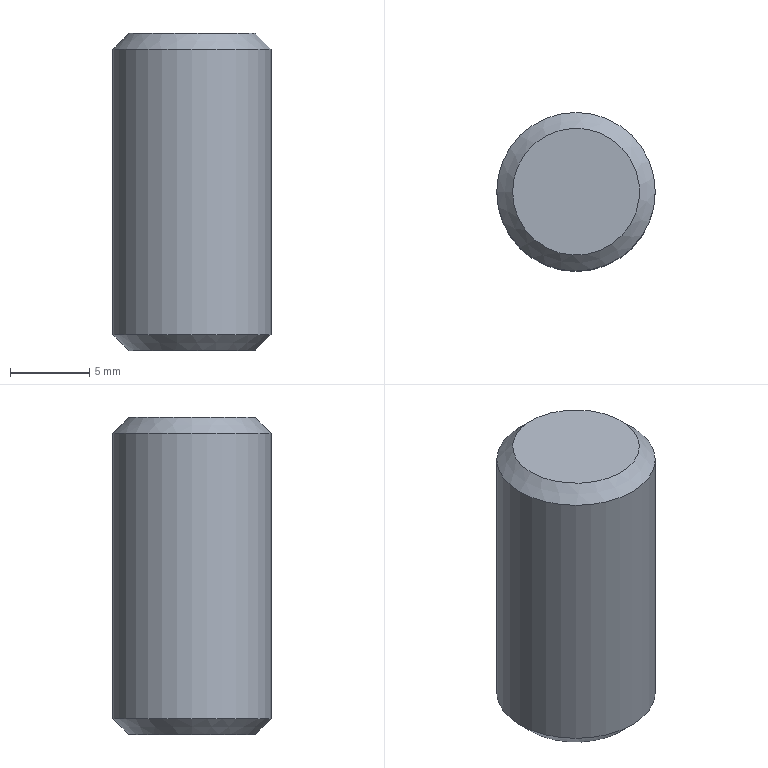Part | NX | features solid 2 | 1 solid | 5 faces | box 10 x 10 x 20 mm | volume 1541 mm3 | plane 2 | cone 2 | cylinder 1 | commonest cylinder face diameters 10 x1
STEP:
#1=CARTESIAN_POINT('',(1320.,-145.,-261.));
#2=VERTEX_POINT('',#1);
#3=CARTESIAN_POINT('',(1325.,-145.,-261.));
#4=DIRECTION('',(0.,0.,-1.));
#5=DIRECTION('',(-1.,0.,0.));
#6=AXIS2_PLACEMENT_3D('',#3,#4,#5);
#7=CIRCLE('',#6,5.);
#8=EDGE_CURVE('',#2,#2,#7,.F.);
#9=ORIENTED_EDGE('',*,*,#8,.F.);
#10=EDGE_LOOP('',(#9));
#11=FACE_BOUND('',#10,.T.);
#12=CARTESIAN_POINT('',(1320.,-145.,-279.));
#13=VERTEX_POINT('',#12);
#14=CARTESIAN_POINT('',(1325.,-145.,-279.));
#15=DIRECTION('',(0.,0.,-1.));
#16=DIRECTION('',(-1.,0.,0.));
#17=AXIS2_PLACEMENT_3D('',#14,#15,#16);
#18=CIRCLE('',#17,5.);
#19=EDGE_CURVE('',#13,#13,#18,.T.);
#20=ORIENTED_EDGE('',*,*,#19,.F.);
#21=EDGE_LOOP('',(#20));
#22=FACE_BOUND('',#21,.T.);
#23=CARTESIAN_POINT('',(1325.,-145.,-280.));
#24=DIRECTION('',(0.,0.,1.));
#25=DIRECTION('',(1.,0.,0.));
#26=AXIS2_PLACEMENT_3D('',#23,#24,#25);
#27=CYLINDRICAL_SURFACE('',#26,5.);
#28=ADVANCED_FACE('',(#11,#22),#27,.T.);
#29=CARTESIAN_POINT('',(1321.,-145.,-280.));
#30=VERTEX_POINT('',#29);
#31=CARTESIAN_POINT('',(1325.,-145.,-280.));
#32=DIRECTION('',(0.,0.,-1.));
#33=DIRECTION('',(-1.,0.,0.));
#34=AXIS2_PLACEMENT_3D('',#31,#32,#33);
#35=CIRCLE('',#34,4.);
#36=EDGE_CURVE('',#30,#30,#35,.F.);
#37=ORIENTED_EDGE('',*,*,#36,.F.);
#38=EDGE_LOOP('',(#37));
#39=FACE_BOUND('',#38,.T.);
#40=CARTESIAN_POINT('',(1325.,-145.,-280.));
#41=DIRECTION('',(0.,0.,1.));
#42=DIRECTION('',(1.,0.,0.));
#43=AXIS2_PLACEMENT_3D('',#40,#41,#42);
#44=PLANE('',#43);
#45=ADVANCED_FACE('',(#39),#44,.F.);
#46=CARTESIAN_POINT('',(1321.,-145.,-260.));
#47=VERTEX_POINT('',#46);
#48=CARTESIAN_POINT('',(1325.,-145.,-260.));
#49=DIRECTION('',(0.,0.,-1.));
#50=DIRECTION('',(-1.,0.,0.));
#51=AXIS2_PLACEMENT_3D('',#48,#49,#50);
#52=CIRCLE('',#51,4.);
#53=EDGE_CURVE('',#47,#47,#52,.T.);
#54=ORIENTED_EDGE('',*,*,#53,.F.);
#55=EDGE_LOOP('',(#54));
#56=FACE_BOUND('',#55,.T.);
#57=CARTESIAN_POINT('',(1325.,-145.,-260.));
#58=DIRECTION('',(0.,0.,1.));
#59=DIRECTION('',(1.,0.,0.));
#60=AXIS2_PLACEMENT_3D('',#57,#58,#59);
#61=PLANE('',#60);
#62=ADVANCED_FACE('',(#56),#61,.T.);
#63=ORIENTED_EDGE('',*,*,#53,.T.);
#64=EDGE_LOOP('',(#63));
#65=FACE_BOUND('',#64,.T.);
#66=ORIENTED_EDGE('',*,*,#8,.T.);
#67=EDGE_LOOP('',(#66));
#68=FACE_BOUND('',#67,.T.);
#69=CARTESIAN_POINT('',(1325.,-145.,-261.));
#70=DIRECTION('',(0.,0.,-1.));
#71=DIRECTION('',(1.,0.,0.));
#72=AXIS2_PLACEMENT_3D('',#69,#70,#71);
#73=CONICAL_SURFACE('',#72,5.,0.7854);
#74=ADVANCED_FACE('',(#65,#68),#73,.T.);
#75=ORIENTED_EDGE('',*,*,#19,.T.);
#76=EDGE_LOOP('',(#75));
#77=FACE_BOUND('',#76,.T.);
#78=ORIENTED_EDGE('',*,*,#36,.T.);
#79=EDGE_LOOP('',(#78));
#80=FACE_BOUND('',#79,.T.);
#81=CARTESIAN_POINT('',(1325.,-145.,-280.));
#82=DIRECTION('',(0.,0.,1.));
#83=DIRECTION('',(-1.,0.,0.));
#84=AXIS2_PLACEMENT_3D('',#81,#82,#83);
#85=CONICAL_SURFACE('',#84,4.,0.7854);
#86=ADVANCED_FACE('',(#77,#80),#85,.T.);
#87=CLOSED_SHELL('',(#28,#45,#62,#74,#86));
#88=MANIFOLD_SOLID_BREP('',#87);
#89=(LENGTH_UNIT()NAMED_UNIT(*)SI_UNIT(.MILLI.,.METRE.));
#90=UNCERTAINTY_MEASURE_WITH_UNIT(LENGTH_MEASURE(0.00001),#89,'','');
#91=(NAMED_UNIT(*)PLANE_ANGLE_UNIT()SI_UNIT($,.RADIAN.));
#92=(NAMED_UNIT(*)SI_UNIT($,.STERADIAN.)SOLID_ANGLE_UNIT());
#93=(GEOMETRIC_REPRESENTATION_CONTEXT(3)GLOBAL_UNCERTAINTY_ASSIGNED_CONTEXT((#90))GLOBAL_UNIT_ASSIGNED_CONTEXT((#89,#91,#92))REPRESENTATION_CONTEXT('',''));
#94=ADVANCED_BREP_SHAPE_REPRESENTATION('',(#88),#93);